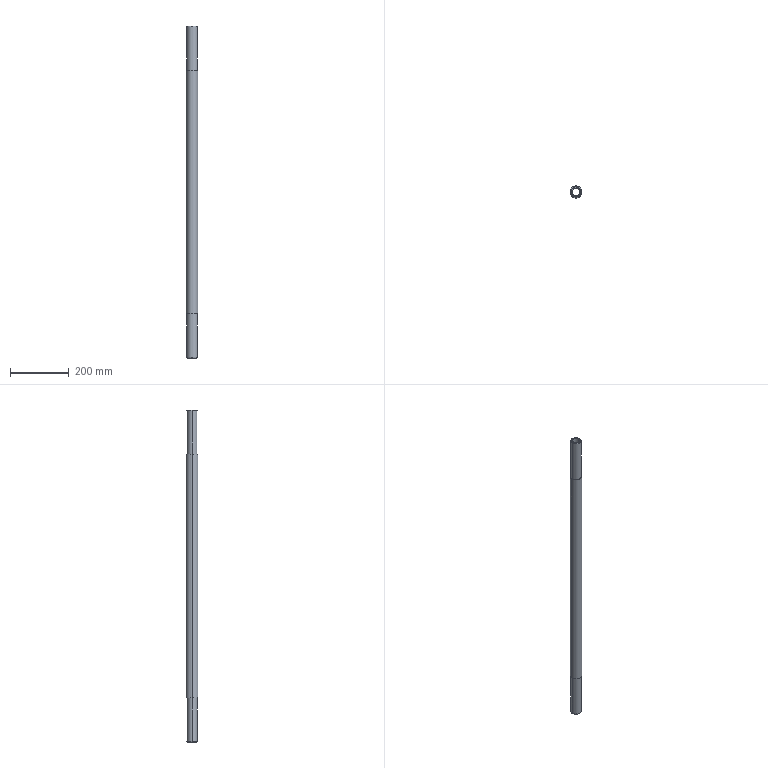Part | STEP file | Roll shaft | 1 solid | 16 faces | box 40 x 40 x 1128 mm | volume 818698 mm3 | cylinder 8 | spline 4 | plane 4 | commonest cylinder face diameters 35 x4 24 x2 40 x2